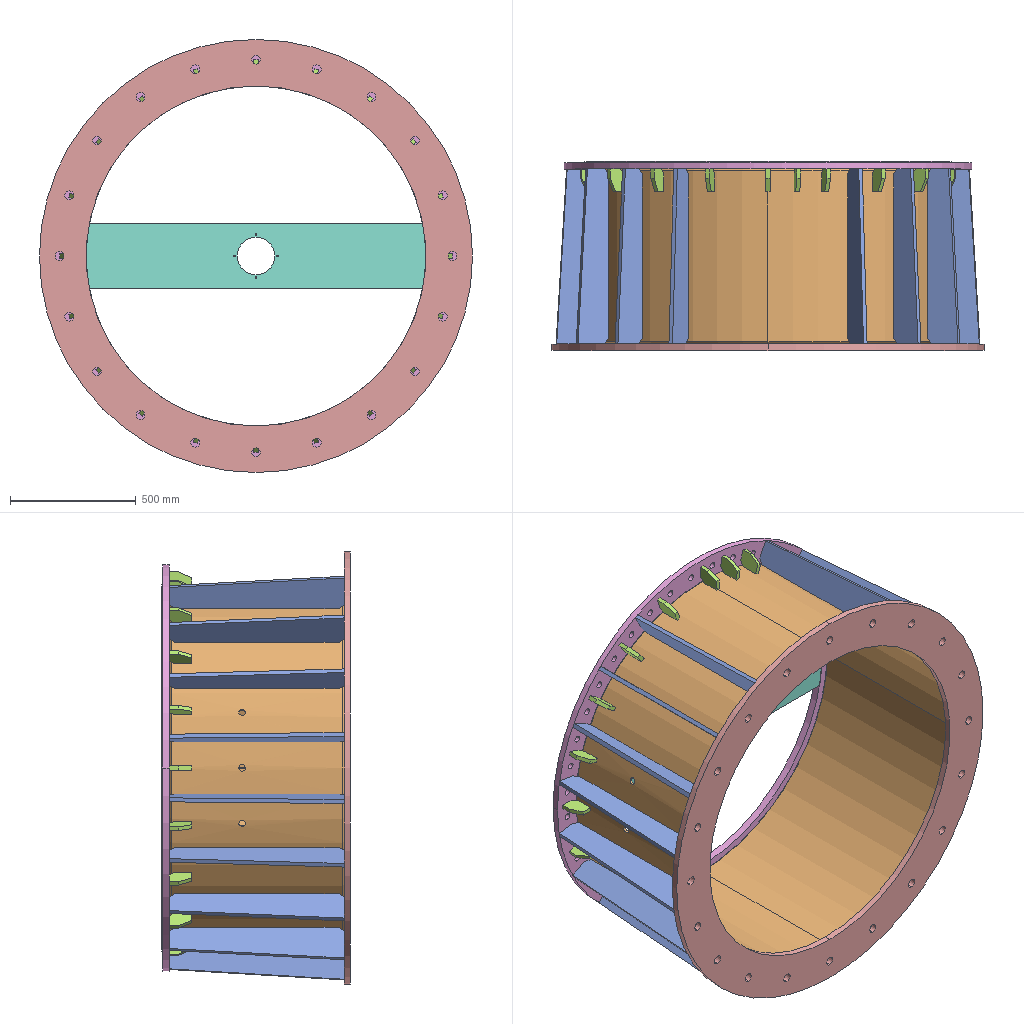Assembly | SolidWorks | 6 different items | 43 placed | box 1720 x 750 x 1720 mm
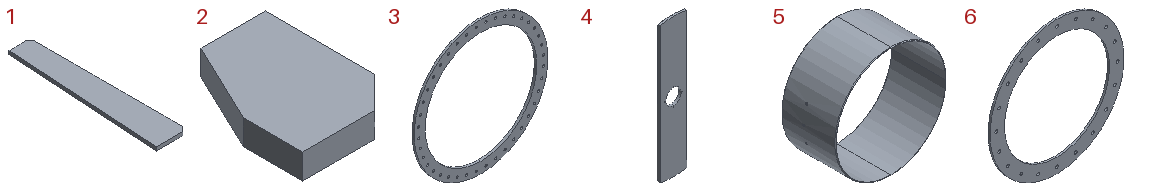Parts list (item | quantity | size | volume | features):
1 | x18 | 137 x 695 x 16 mm | 1283520 mm3 | features Chamfer 1, Extrusion 1
2 | x21 | 66 x 90 x 16 mm | 81440 mm3 | features Chamfer 1, Extrusion 1
3 | x1 | 1620 x 30 x 1620 mm | 16428173 mm3 | features ICE 4, HoleWzd 2, Extrusion 1
4 | x1 | 260 x 30 x 1350 mm | 9802887 mm3 | features ICE 4, HoleWzd 2, Chamfer 1, Extrusion 1
5 | x1 | 1428 x 695 x 1428 mm | 30589122 mm3 | features Chamfer 2, CirPattern 2, FlatPattern 1, HoleWzd 1, SMBaseFlange 1, SheetMetal 1
6 | x1 | 1720 x 25 x 1720 mm | 21822288 mm3 | features Extrusion 1, HoleWzd 1
Mates (type | each side: item.copy, entity, surface, feature):
Concentric | 6.1 face cylinder Boss-Extrude 1 | 5.1 face cylinder BaseBend1
Concentric | 3.1 face cylinder Boss-Extrude 1 | 5.1 face cylinder BaseBend1
Coincident | 6.1 face plane Boss-Extrude 1 | 5.1 face plane BaseBend1
Coincident | 3.1 face plane Boss-Extrude 1 | 5.1 face plane BaseBend1
Perpendicular | 3.1 plane | assembly plane
Coincident | 5.1 plane | assembly plane
Coincident | 6.1 face plane Boss-Extrude 1 | 1.1 face plane Boss-Extrude 1
Coincident | 1.1 plane | assembly select_type:10
Tangent | 1.1 face plane Boss-Extrude 1 | 5.1 face cylinder BaseBend1
Coincident | 2.1 plane | assembly plane
Coordinate | 6.1 select_type:25 | assembly select_type:11
Coincident | 2.1 face plane Boss-Extrude 1 | 3.1 face plane Boss-Extrude 1
Tangent | 2.1 face plane Boss-Extrude 1 | 5.1 face cylinder BaseBend1
Coincident | 3.1 face plane Boss-Extrude 2 | 4.1 face plane Boss-Extrude 2
Coincident | 4.1 plane | assembly plane
Concentric | 3.1 face cylinder Cut-Extrude 1 | 4.1 face cylinder Cut-Extrude 3